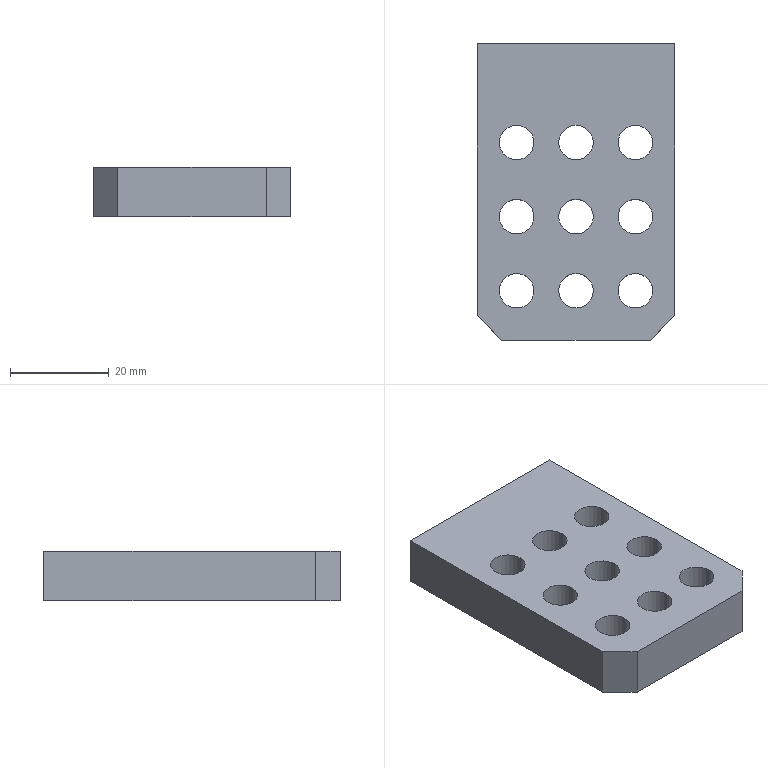Part | STEP file | PN_0077 Mount electronic clip suction nozzle mounting plate | 1 solid | 34 faces | box 40 x 60 x 10 mm | volume 19887 mm3 | cylinder 22 | plane 8 | cone 4 | commonest cylinder face diameters 7 x18 4.2 x4